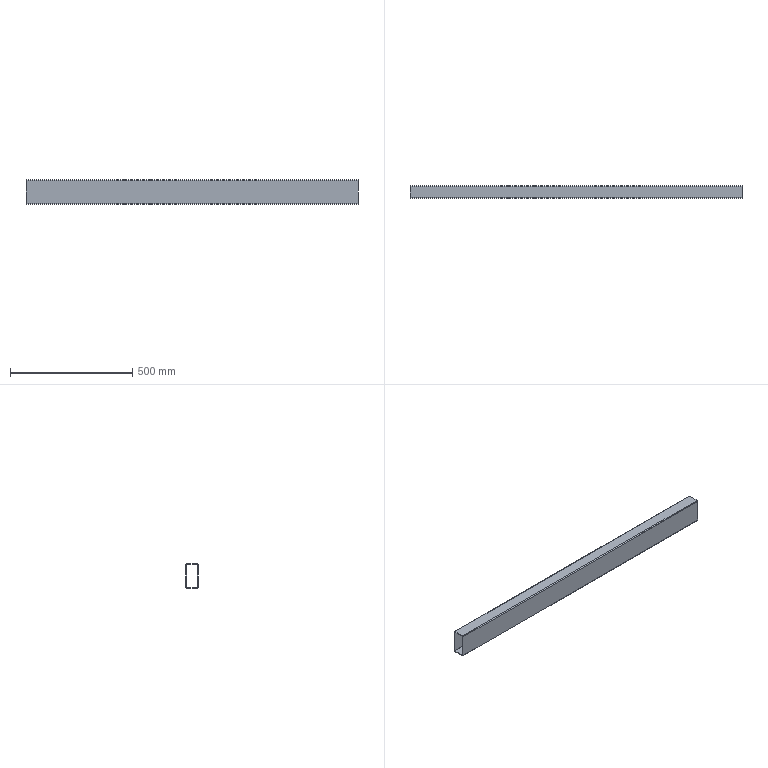Part | SolidWorks | features BaseBody 1, MoveFace 1 | 1 solid | 18 faces | box 1356 x 50 x 100 mm | volume 1157616 mm3 | plane 10 | cylinder 8 | commonest cylinder face diameters 1 x4 7 x4
STEP:
#1=CARTESIAN_POINT('',(976.,21.5,-50.));
#2=VERTEX_POINT('',#1);
#3=CARTESIAN_POINT('',(976.,25.,-46.5));
#4=VERTEX_POINT('',#3);
#5=CARTESIAN_POINT('',(976.,21.5,-46.5));
#6=DIRECTION('',(1.,0.,0.));
#7=DIRECTION('',(0.,0.,1.));
#8=AXIS2_PLACEMENT_3D('',#5,#6,#7);
#9=CIRCLE('',#8,3.5);
#10=EDGE_CURVE('',#2,#4,#9,.T.);
#11=ORIENTED_EDGE('',*,*,#10,.T.);
#12=CARTESIAN_POINT('',(976.,25.,46.5));
#13=VERTEX_POINT('',#12);
#14=CARTESIAN_POINT('',(976.,25.,46.5));
#15=DIRECTION('',(0.,0.,1.));
#16=VECTOR('',#15,1000.);
#17=LINE('',#14,#16);
#18=EDGE_CURVE('',#4,#13,#17,.T.);
#19=ORIENTED_EDGE('',*,*,#18,.T.);
#20=CARTESIAN_POINT('',(976.,21.5,50.));
#21=VERTEX_POINT('',#20);
#22=CARTESIAN_POINT('',(976.,21.5,46.5));
#23=DIRECTION('',(1.,0.,0.));
#24=DIRECTION('',(0.,0.,-1.));
#25=AXIS2_PLACEMENT_3D('',#22,#23,#24);
#26=CIRCLE('',#25,3.5);
#27=EDGE_CURVE('',#13,#21,#26,.T.);
#28=ORIENTED_EDGE('',*,*,#27,.T.);
#29=CARTESIAN_POINT('',(976.,-21.5,50.));
#30=VERTEX_POINT('',#29);
#31=CARTESIAN_POINT('',(976.,21.5,50.));
#32=DIRECTION('',(0.,-1.,0.));
#33=VECTOR('',#32,1000.);
#34=LINE('',#31,#33);
#35=EDGE_CURVE('',#21,#30,#34,.T.);
#36=ORIENTED_EDGE('',*,*,#35,.T.);
#37=CARTESIAN_POINT('',(976.,-25.,46.5));
#38=VERTEX_POINT('',#37);
#39=CARTESIAN_POINT('',(976.,-21.5,46.5));
#40=DIRECTION('',(1.,0.,0.));
#41=DIRECTION('',(0.,0.,-1.));
#42=AXIS2_PLACEMENT_3D('',#39,#40,#41);
#43=CIRCLE('',#42,3.5);
#44=EDGE_CURVE('',#30,#38,#43,.T.);
#45=ORIENTED_EDGE('',*,*,#44,.T.);
#46=CARTESIAN_POINT('',(976.,-25.,-46.5));
#47=VERTEX_POINT('',#46);
#48=CARTESIAN_POINT('',(976.,-25.,46.5));
#49=DIRECTION('',(0.,0.,-1.));
#50=VECTOR('',#49,1000.);
#51=LINE('',#48,#50);
#52=EDGE_CURVE('',#38,#47,#51,.T.);
#53=ORIENTED_EDGE('',*,*,#52,.T.);
#54=CARTESIAN_POINT('',(976.,-21.5,-50.));
#55=VERTEX_POINT('',#54);
#56=CARTESIAN_POINT('',(976.,-21.5,-46.5));
#57=DIRECTION('',(1.,0.,0.));
#58=DIRECTION('',(0.,0.,-1.));
#59=AXIS2_PLACEMENT_3D('',#56,#57,#58);
#60=CIRCLE('',#59,3.5);
#61=EDGE_CURVE('',#47,#55,#60,.T.);
#62=ORIENTED_EDGE('',*,*,#61,.T.);
#63=CARTESIAN_POINT('',(976.,21.5,-50.));
#64=DIRECTION('',(0.,1.,0.));
#65=VECTOR('',#64,1000.);
#66=LINE('',#63,#65);
#67=EDGE_CURVE('',#55,#2,#66,.T.);
#68=ORIENTED_EDGE('',*,*,#67,.T.);
#69=EDGE_LOOP('',(#11,#19,#28,#36,#45,#53,#62,#68));
#70=FACE_OUTER_BOUND('',#69,.T.);
#71=CARTESIAN_POINT('',(976.,22.,-46.5));
#72=VERTEX_POINT('',#71);
#73=CARTESIAN_POINT('',(976.,22.,46.5));
#74=VERTEX_POINT('',#73);
#75=CARTESIAN_POINT('',(976.,22.,-46.5));
#76=DIRECTION('',(0.,0.,1.));
#77=VECTOR('',#76,1000.);
#78=LINE('',#75,#77);
#79=EDGE_CURVE('',#72,#74,#78,.T.);
#80=ORIENTED_EDGE('',*,*,#79,.F.);
#81=CARTESIAN_POINT('',(976.,21.5,-47.));
#82=VERTEX_POINT('',#81);
#83=CARTESIAN_POINT('',(976.,21.5,-46.5));
#84=DIRECTION('',(1.,0.,0.));
#85=DIRECTION('',(0.,0.,1.));
#86=AXIS2_PLACEMENT_3D('',#83,#84,#85);
#87=CIRCLE('',#86,0.5);
#88=EDGE_CURVE('',#82,#72,#87,.T.);
#89=ORIENTED_EDGE('',*,*,#88,.F.);
#90=CARTESIAN_POINT('',(976.,-21.5,-47.));
#91=VERTEX_POINT('',#90);
#92=CARTESIAN_POINT('',(976.,21.5,-47.));
#93=DIRECTION('',(0.,1.,0.));
#94=VECTOR('',#93,1000.);
#95=LINE('',#92,#94);
#96=EDGE_CURVE('',#91,#82,#95,.T.);
#97=ORIENTED_EDGE('',*,*,#96,.F.);
#98=CARTESIAN_POINT('',(976.,-22.,-46.5));
#99=VERTEX_POINT('',#98);
#100=CARTESIAN_POINT('',(976.,-21.5,-46.5));
#101=DIRECTION('',(1.,0.,0.));
#102=DIRECTION('',(0.,0.,1.));
#103=AXIS2_PLACEMENT_3D('',#100,#101,#102);
#104=CIRCLE('',#103,0.5);
#105=EDGE_CURVE('',#99,#91,#104,.T.);
#106=ORIENTED_EDGE('',*,*,#105,.F.);
#107=CARTESIAN_POINT('',(976.,-22.,46.5));
#108=VERTEX_POINT('',#107);
#109=CARTESIAN_POINT('',(976.,-22.,-46.5));
#110=DIRECTION('',(0.,0.,-1.));
#111=VECTOR('',#110,1000.);
#112=LINE('',#109,#111);
#113=EDGE_CURVE('',#108,#99,#112,.T.);
#114=ORIENTED_EDGE('',*,*,#113,.F.);
#115=CARTESIAN_POINT('',(976.,-21.5,47.));
#116=VERTEX_POINT('',#115);
#117=CARTESIAN_POINT('',(976.,-21.5,46.5));
#118=DIRECTION('',(1.,0.,0.));
#119=DIRECTION('',(0.,0.,1.));
#120=AXIS2_PLACEMENT_3D('',#117,#118,#119);
#121=CIRCLE('',#120,0.5);
#122=EDGE_CURVE('',#116,#108,#121,.T.);
#123=ORIENTED_EDGE('',*,*,#122,.F.);
#124=CARTESIAN_POINT('',(976.,21.5,47.));
#125=VERTEX_POINT('',#124);
#126=CARTESIAN_POINT('',(976.,21.5,47.));
#127=DIRECTION('',(0.,-1.,0.));
#128=VECTOR('',#127,1000.);
#129=LINE('',#126,#128);
#130=EDGE_CURVE('',#125,#116,#129,.T.);
#131=ORIENTED_EDGE('',*,*,#130,.F.);
#132=CARTESIAN_POINT('',(976.,21.5,46.5));
#133=DIRECTION('',(1.,0.,0.));
#134=DIRECTION('',(0.,0.,1.));
#135=AXIS2_PLACEMENT_3D('',#132,#133,#134);
#136=CIRCLE('',#135,0.5);
#137=EDGE_CURVE('',#74,#125,#136,.T.);
#138=ORIENTED_EDGE('',*,*,#137,.F.);
#139=EDGE_LOOP('',(#80,#89,#97,#106,#114,#123,#131,#138));
#140=FACE_BOUND('',#139,.T.);
#141=CARTESIAN_POINT('',(976.,21.5,-46.5));
#142=DIRECTION('',(1.,0.,0.));
#143=DIRECTION('',(0.,0.,-1.));
#144=AXIS2_PLACEMENT_3D('',#141,#142,#143);
#145=PLANE('',#144);
#146=ADVANCED_FACE('',(#70,#140),#145,.T.);
#147=CARTESIAN_POINT('',(-380.,21.5,-50.));
#148=VERTEX_POINT('',#147);
#149=CARTESIAN_POINT('',(-380.,25.,-46.5));
#150=VERTEX_POINT('',#149);
#151=CARTESIAN_POINT('',(-380.,21.5,-46.5));
#152=DIRECTION('',(1.,0.,0.));
#153=DIRECTION('',(0.,0.,1.));
#154=AXIS2_PLACEMENT_3D('',#151,#152,#153);
#155=CIRCLE('',#154,3.5);
#156=EDGE_CURVE('',#148,#150,#155,.T.);
#157=ORIENTED_EDGE('',*,*,#156,.F.);
#158=CARTESIAN_POINT('',(-380.,-21.5,-50.));
#159=VERTEX_POINT('',#158);
#160=CARTESIAN_POINT('',(-380.,21.5,-50.));
#161=DIRECTION('',(0.,1.,0.));
#162=VECTOR('',#161,1000.);
#163=LINE('',#160,#162);
#164=EDGE_CURVE('',#159,#148,#163,.T.);
#165=ORIENTED_EDGE('',*,*,#164,.F.);
#166=CARTESIAN_POINT('',(-380.,-25.,-46.5));
#167=VERTEX_POINT('',#166);
#168=CARTESIAN_POINT('',(-380.,-21.5,-46.5));
#169=DIRECTION('',(1.,0.,0.));
#170=DIRECTION('',(0.,0.,-1.));
#171=AXIS2_PLACEMENT_3D('',#168,#169,#170);
#172=CIRCLE('',#171,3.5);
#173=EDGE_CURVE('',#167,#159,#172,.T.);
#174=ORIENTED_EDGE('',*,*,#173,.F.);
#175=CARTESIAN_POINT('',(-380.,-25.,46.5));
#176=VERTEX_POINT('',#175);
#177=CARTESIAN_POINT('',(-380.,-25.,46.5));
#178=DIRECTION('',(0.,0.,-1.));
#179=VECTOR('',#178,1000.);
#180=LINE('',#177,#179);
#181=EDGE_CURVE('',#176,#167,#180,.T.);
#182=ORIENTED_EDGE('',*,*,#181,.F.);
#183=CARTESIAN_POINT('',(-380.,-21.5,50.));
#184=VERTEX_POINT('',#183);
#185=CARTESIAN_POINT('',(-380.,-21.5,46.5));
#186=DIRECTION('',(1.,0.,0.));
#187=DIRECTION('',(0.,0.,-1.));
#188=AXIS2_PLACEMENT_3D('',#185,#186,#187);
#189=CIRCLE('',#188,3.5);
#190=EDGE_CURVE('',#184,#176,#189,.T.);
#191=ORIENTED_EDGE('',*,*,#190,.F.);
#192=CARTESIAN_POINT('',(-380.,21.5,50.));
#193=VERTEX_POINT('',#192);
#194=CARTESIAN_POINT('',(-380.,21.5,50.));
#195=DIRECTION('',(0.,-1.,0.));
#196=VECTOR('',#195,1000.);
#197=LINE('',#194,#196);
#198=EDGE_CURVE('',#193,#184,#197,.T.);
#199=ORIENTED_EDGE('',*,*,#198,.F.);
#200=CARTESIAN_POINT('',(-380.,25.,46.5));
#201=VERTEX_POINT('',#200);
#202=CARTESIAN_POINT('',(-380.,21.5,46.5));
#203=DIRECTION('',(1.,0.,0.));
#204=DIRECTION('',(0.,0.,-1.));
#205=AXIS2_PLACEMENT_3D('',#202,#203,#204);
#206=CIRCLE('',#205,3.5);
#207=EDGE_CURVE('',#201,#193,#206,.T.);
#208=ORIENTED_EDGE('',*,*,#207,.F.);
#209=CARTESIAN_POINT('',(-380.,25.,46.5));
#210=DIRECTION('',(0.,0.,1.));
#211=VECTOR('',#210,1000.);
#212=LINE('',#209,#211);
#213=EDGE_CURVE('',#150,#201,#212,.T.);
#214=ORIENTED_EDGE('',*,*,#213,.F.);
#215=EDGE_LOOP('',(#157,#165,#174,#182,#191,#199,#208,#214));
#216=FACE_OUTER_BOUND('',#215,.T.);
#217=CARTESIAN_POINT('',(-380.,21.5,-47.));
#218=VERTEX_POINT('',#217);
#219=CARTESIAN_POINT('',(-380.,22.,-46.5));
#220=VERTEX_POINT('',#219);
#221=CARTESIAN_POINT('',(-380.,21.5,-46.5));
#222=DIRECTION('',(1.,0.,0.));
#223=DIRECTION('',(0.,0.,1.));
#224=AXIS2_PLACEMENT_3D('',#221,#222,#223);
#225=CIRCLE('',#224,0.5);
#226=EDGE_CURVE('',#218,#220,#225,.T.);
#227=ORIENTED_EDGE('',*,*,#226,.T.);
#228=CARTESIAN_POINT('',(-380.,22.,46.5));
#229=VERTEX_POINT('',#228);
#230=CARTESIAN_POINT('',(-380.,22.,-46.5));
#231=DIRECTION('',(0.,0.,1.));
#232=VECTOR('',#231,1000.);
#233=LINE('',#230,#232);
#234=EDGE_CURVE('',#220,#229,#233,.T.);
#235=ORIENTED_EDGE('',*,*,#234,.T.);
#236=CARTESIAN_POINT('',(-380.,21.5,47.));
#237=VERTEX_POINT('',#236);
#238=CARTESIAN_POINT('',(-380.,21.5,46.5));
#239=DIRECTION('',(1.,0.,0.));
#240=DIRECTION('',(0.,0.,1.));
#241=AXIS2_PLACEMENT_3D('',#238,#239,#240);
#242=CIRCLE('',#241,0.5);
#243=EDGE_CURVE('',#229,#237,#242,.T.);
#244=ORIENTED_EDGE('',*,*,#243,.T.);
#245=CARTESIAN_POINT('',(-380.,-21.5,47.));
#246=VERTEX_POINT('',#245);
#247=CARTESIAN_POINT('',(-380.,21.5,47.));
#248=DIRECTION('',(0.,-1.,0.));
#249=VECTOR('',#248,1000.);
#250=LINE('',#247,#249);
#251=EDGE_CURVE('',#237,#246,#250,.T.);
#252=ORIENTED_EDGE('',*,*,#251,.T.);
#253=CARTESIAN_POINT('',(-380.,-22.,46.5));
#254=VERTEX_POINT('',#253);
#255=CARTESIAN_POINT('',(-380.,-21.5,46.5));
#256=DIRECTION('',(1.,0.,0.));
#257=DIRECTION('',(0.,0.,1.));
#258=AXIS2_PLACEMENT_3D('',#255,#256,#257);
#259=CIRCLE('',#258,0.5);
#260=EDGE_CURVE('',#246,#254,#259,.T.);
#261=ORIENTED_EDGE('',*,*,#260,.T.);
#262=CARTESIAN_POINT('',(-380.,-22.,-46.5));
#263=VERTEX_POINT('',#262);
#264=CARTESIAN_POINT('',(-380.,-22.,-46.5));
#265=DIRECTION('',(0.,0.,-1.));
#266=VECTOR('',#265,1000.);
#267=LINE('',#264,#266);
#268=EDGE_CURVE('',#254,#263,#267,.T.);
#269=ORIENTED_EDGE('',*,*,#268,.T.);
#270=CARTESIAN_POINT('',(-380.,-21.5,-47.));
#271=VERTEX_POINT('',#270);
#272=CARTESIAN_POINT('',(-380.,-21.5,-46.5));
#273=DIRECTION('',(1.,0.,0.));
#274=DIRECTION('',(0.,0.,1.));
#275=AXIS2_PLACEMENT_3D('',#272,#273,#274);
#276=CIRCLE('',#275,0.5);
#277=EDGE_CURVE('',#263,#271,#276,.T.);
#278=ORIENTED_EDGE('',*,*,#277,.T.);
#279=CARTESIAN_POINT('',(-380.,21.5,-47.));
#280=DIRECTION('',(0.,1.,0.));
#281=VECTOR('',#280,1000.);
#282=LINE('',#279,#281);
#283=EDGE_CURVE('',#271,#218,#282,.T.);
#284=ORIENTED_EDGE('',*,*,#283,.T.);
#285=EDGE_LOOP('',(#227,#235,#244,#252,#261,#269,#278,#284));
#286=FACE_BOUND('',#285,.T.);
#287=CARTESIAN_POINT('',(-380.,21.5,-46.5));
#288=DIRECTION('',(1.,0.,0.));
#289=DIRECTION('',(0.,0.,-1.));
#290=AXIS2_PLACEMENT_3D('',#287,#288,#289);
#291=PLANE('',#290);
#292=ADVANCED_FACE('',(#216,#286),#291,.F.);
#293=ORIENTED_EDGE('',*,*,#156,.T.);
#294=CARTESIAN_POINT('',(976.,25.,-46.5));
#295=DIRECTION('',(-1.,0.,0.));
#296=VECTOR('',#295,1000.);
#297=LINE('',#294,#296);
#298=EDGE_CURVE('',#4,#150,#297,.T.);
#299=ORIENTED_EDGE('',*,*,#298,.F.);
#300=ORIENTED_EDGE('',*,*,#10,.F.);
#301=CARTESIAN_POINT('',(976.,21.5,-50.));
#302=DIRECTION('',(-1.,0.,0.));
#303=VECTOR('',#302,1000.);
#304=LINE('',#301,#303);
#305=EDGE_CURVE('',#2,#148,#304,.T.);
#306=ORIENTED_EDGE('',*,*,#305,.T.);
#307=EDGE_LOOP('',(#293,#299,#300,#306));
#308=FACE_OUTER_BOUND('',#307,.T.);
#309=CARTESIAN_POINT('',(976.,21.5,-46.5));
#310=DIRECTION('',(-1.,0.,0.));
#311=DIRECTION('',(0.,0.,1.));
#312=AXIS2_PLACEMENT_3D('',#309,#310,#311);
#313=CYLINDRICAL_SURFACE('',#312,3.5);
#314=ADVANCED_FACE('',(#308),#313,.T.);
#315=ORIENTED_EDGE('',*,*,#213,.T.);
#316=CARTESIAN_POINT('',(976.,25.,46.5));
#317=DIRECTION('',(-1.,0.,0.));
#318=VECTOR('',#317,1000.);
#319=LINE('',#316,#318);
#320=EDGE_CURVE('',#13,#201,#319,.T.);
#321=ORIENTED_EDGE('',*,*,#320,.F.);
#322=ORIENTED_EDGE('',*,*,#18,.F.);
#323=ORIENTED_EDGE('',*,*,#298,.T.);
#324=EDGE_LOOP('',(#315,#321,#322,#323));
#325=FACE_OUTER_BOUND('',#324,.T.);
#326=CARTESIAN_POINT('',(976.,25.,46.5));
#327=DIRECTION('',(0.,-1.,0.));
#328=DIRECTION('',(0.,0.,-1.));
#329=AXIS2_PLACEMENT_3D('',#326,#327,#328);
#330=PLANE('',#329);
#331=ADVANCED_FACE('',(#325),#330,.F.);
#332=ORIENTED_EDGE('',*,*,#207,.T.);
#333=CARTESIAN_POINT('',(976.,21.5,50.));
#334=DIRECTION('',(-1.,0.,0.));
#335=VECTOR('',#334,1000.);
#336=LINE('',#333,#335);
#337=EDGE_CURVE('',#21,#193,#336,.T.);
#338=ORIENTED_EDGE('',*,*,#337,.F.);
#339=ORIENTED_EDGE('',*,*,#27,.F.);
#340=ORIENTED_EDGE('',*,*,#320,.T.);
#341=EDGE_LOOP('',(#332,#338,#339,#340));
#342=FACE_OUTER_BOUND('',#341,.T.);
#343=CARTESIAN_POINT('',(976.,21.5,46.5));
#344=DIRECTION('',(-1.,0.,0.));
#345=DIRECTION('',(0.,0.,1.));
#346=AXIS2_PLACEMENT_3D('',#343,#344,#345);
#347=CYLINDRICAL_SURFACE('',#346,3.5);
#348=ADVANCED_FACE('',(#342),#347,.T.);
#349=ORIENTED_EDGE('',*,*,#198,.T.);
#350=CARTESIAN_POINT('',(976.,-21.5,50.));
#351=DIRECTION('',(-1.,0.,0.));
#352=VECTOR('',#351,1000.);
#353=LINE('',#350,#352);
#354=EDGE_CURVE('',#30,#184,#353,.T.);
#355=ORIENTED_EDGE('',*,*,#354,.F.);
#356=ORIENTED_EDGE('',*,*,#35,.F.);
#357=ORIENTED_EDGE('',*,*,#337,.T.);
#358=EDGE_LOOP('',(#349,#355,#356,#357));
#359=FACE_OUTER_BOUND('',#358,.T.);
#360=CARTESIAN_POINT('',(976.,21.5,50.));
#361=DIRECTION('',(0.,0.,-1.));
#362=DIRECTION('',(-1.,0.,0.));
#363=AXIS2_PLACEMENT_3D('',#360,#361,#362);
#364=PLANE('',#363);
#365=ADVANCED_FACE('',(#359),#364,.F.);
#366=ORIENTED_EDGE('',*,*,#190,.T.);
#367=CARTESIAN_POINT('',(976.,-25.,46.5));
#368=DIRECTION('',(-1.,0.,0.));
#369=VECTOR('',#368,1000.);
#370=LINE('',#367,#369);
#371=EDGE_CURVE('',#38,#176,#370,.T.);
#372=ORIENTED_EDGE('',*,*,#371,.F.);
#373=ORIENTED_EDGE('',*,*,#44,.F.);
#374=ORIENTED_EDGE('',*,*,#354,.T.);
#375=EDGE_LOOP('',(#366,#372,#373,#374));
#376=FACE_OUTER_BOUND('',#375,.T.);
#377=CARTESIAN_POINT('',(976.,-21.5,46.5));
#378=DIRECTION('',(-1.,0.,0.));
#379=DIRECTION('',(0.,0.,1.));
#380=AXIS2_PLACEMENT_3D('',#377,#378,#379);
#381=CYLINDRICAL_SURFACE('',#380,3.5);
#382=ADVANCED_FACE('',(#376),#381,.T.);
#383=ORIENTED_EDGE('',*,*,#181,.T.);
#384=CARTESIAN_POINT('',(976.,-25.,-46.5));
#385=DIRECTION('',(-1.,0.,0.));
#386=VECTOR('',#385,1000.);
#387=LINE('',#384,#386);
#388=EDGE_CURVE('',#47,#167,#387,.T.);
#389=ORIENTED_EDGE('',*,*,#388,.F.);
#390=ORIENTED_EDGE('',*,*,#52,.F.);
#391=ORIENTED_EDGE('',*,*,#371,.T.);
#392=EDGE_LOOP('',(#383,#389,#390,#391));
#393=FACE_OUTER_BOUND('',#392,.T.);
#394=CARTESIAN_POINT('',(976.,-25.,46.5));
#395=DIRECTION('',(0.,1.,0.));
#396=DIRECTION('',(0.,0.,1.));
#397=AXIS2_PLACEMENT_3D('',#394,#395,#396);
#398=PLANE('',#397);
#399=ADVANCED_FACE('',(#393),#398,.F.);
#400=ORIENTED_EDGE('',*,*,#173,.T.);
#401=CARTESIAN_POINT('',(976.,-21.5,-50.));
#402=DIRECTION('',(-1.,0.,0.));
#403=VECTOR('',#402,1000.);
#404=LINE('',#401,#403);
#405=EDGE_CURVE('',#55,#159,#404,.T.);
#406=ORIENTED_EDGE('',*,*,#405,.F.);
#407=ORIENTED_EDGE('',*,*,#61,.F.);
#408=ORIENTED_EDGE('',*,*,#388,.T.);
#409=EDGE_LOOP('',(#400,#406,#407,#408));
#410=FACE_OUTER_BOUND('',#409,.T.);
#411=CARTESIAN_POINT('',(976.,-21.5,-46.5));
#412=DIRECTION('',(-1.,0.,0.));
#413=DIRECTION('',(0.,0.,1.));
#414=AXIS2_PLACEMENT_3D('',#411,#412,#413);
#415=CYLINDRICAL_SURFACE('',#414,3.5);
#416=ADVANCED_FACE('',(#410),#415,.T.);
#417=ORIENTED_EDGE('',*,*,#164,.T.);
#418=ORIENTED_EDGE('',*,*,#305,.F.);
#419=ORIENTED_EDGE('',*,*,#67,.F.);
#420=ORIENTED_EDGE('',*,*,#405,.T.);
#421=EDGE_LOOP('',(#417,#418,#419,#420));
#422=FACE_OUTER_BOUND('',#421,.T.);
#423=CARTESIAN_POINT('',(976.,21.5,-50.));
#424=DIRECTION('',(0.,0.,1.));
#425=DIRECTION('',(0.,-1.,0.));
#426=AXIS2_PLACEMENT_3D('',#423,#424,#425);
#427=PLANE('',#426);
#428=ADVANCED_FACE('',(#422),#427,.F.);
#429=ORIENTED_EDGE('',*,*,#226,.F.);
#430=CARTESIAN_POINT('',(976.,21.5,-47.));
#431=DIRECTION('',(-1.,0.,0.));
#432=VECTOR('',#431,1000.);
#433=LINE('',#430,#432);
#434=EDGE_CURVE('',#82,#218,#433,.T.);
#435=ORIENTED_EDGE('',*,*,#434,.F.);
#436=ORIENTED_EDGE('',*,*,#88,.T.);
#437=CARTESIAN_POINT('',(976.,22.,-46.5));
#438=DIRECTION('',(-1.,0.,0.));
#439=VECTOR('',#438,1000.);
#440=LINE('',#437,#439);
#441=EDGE_CURVE('',#72,#220,#440,.T.);
#442=ORIENTED_EDGE('',*,*,#441,.T.);
#443=EDGE_LOOP('',(#429,#435,#436,#442));
#444=FACE_OUTER_BOUND('',#443,.T.);
#445=CARTESIAN_POINT('',(976.,21.5,-46.5));
#446=DIRECTION('',(-1.,0.,0.));
#447=DIRECTION('',(0.,0.,1.));
#448=AXIS2_PLACEMENT_3D('',#445,#446,#447);
#449=CYLINDRICAL_SURFACE('',#448,0.5);
#450=ADVANCED_FACE('',(#444),#449,.F.);
#451=ORIENTED_EDGE('',*,*,#234,.F.);
#452=ORIENTED_EDGE('',*,*,#441,.F.);
#453=ORIENTED_EDGE('',*,*,#79,.T.);
#454=CARTESIAN_POINT('',(976.,22.,46.5));
#455=DIRECTION('',(-1.,0.,0.));
#456=VECTOR('',#455,1000.);
#457=LINE('',#454,#456);
#458=EDGE_CURVE('',#74,#229,#457,.T.);
#459=ORIENTED_EDGE('',*,*,#458,.T.);
#460=EDGE_LOOP('',(#451,#452,#453,#459));
#461=FACE_OUTER_BOUND('',#460,.T.);
#462=CARTESIAN_POINT('',(976.,22.,-46.5));
#463=DIRECTION('',(0.,-1.,0.));
#464=DIRECTION('',(0.,0.,-1.));
#465=AXIS2_PLACEMENT_3D('',#462,#463,#464);
#466=PLANE('',#465);
#467=ADVANCED_FACE('',(#461),#466,.T.);
#468=ORIENTED_EDGE('',*,*,#243,.F.);
#469=ORIENTED_EDGE('',*,*,#458,.F.);
#470=ORIENTED_EDGE('',*,*,#137,.T.);
#471=CARTESIAN_POINT('',(976.,21.5,47.));
#472=DIRECTION('',(-1.,0.,0.));
#473=VECTOR('',#472,1000.);
#474=LINE('',#471,#473);
#475=EDGE_CURVE('',#125,#237,#474,.T.);
#476=ORIENTED_EDGE('',*,*,#475,.T.);
#477=EDGE_LOOP('',(#468,#469,#470,#476));
#478=FACE_OUTER_BOUND('',#477,.T.);
#479=CARTESIAN_POINT('',(976.,21.5,46.5));
#480=DIRECTION('',(-1.,0.,0.));
#481=DIRECTION('',(0.,0.,1.));
#482=AXIS2_PLACEMENT_3D('',#479,#480,#481);
#483=CYLINDRICAL_SURFACE('',#482,0.5);
#484=ADVANCED_FACE('',(#478),#483,.F.);
#485=ORIENTED_EDGE('',*,*,#251,.F.);
#486=ORIENTED_EDGE('',*,*,#475,.F.);
#487=ORIENTED_EDGE('',*,*,#130,.T.);
#488=CARTESIAN_POINT('',(976.,-21.5,47.));
#489=DIRECTION('',(-1.,0.,0.));
#490=VECTOR('',#489,1000.);
#491=LINE('',#488,#490);
#492=EDGE_CURVE('',#116,#246,#491,.T.);
#493=ORIENTED_EDGE('',*,*,#492,.T.);
#494=EDGE_LOOP('',(#485,#486,#487,#493));
#495=FACE_OUTER_BOUND('',#494,.T.);
#496=CARTESIAN_POINT('',(976.,21.5,47.));
#497=DIRECTION('',(0.,0.,-1.));
#498=DIRECTION('',(-1.,0.,0.));
#499=AXIS2_PLACEMENT_3D('',#496,#497,#498);
#500=PLANE('',#499);
#501=ADVANCED_FACE('',(#495),#500,.T.);
#502=ORIENTED_EDGE('',*,*,#260,.F.);
#503=ORIENTED_EDGE('',*,*,#492,.F.);
#504=ORIENTED_EDGE('',*,*,#122,.T.);
#505=CARTESIAN_POINT('',(976.,-22.,46.5));
#506=DIRECTION('',(-1.,0.,0.));
#507=VECTOR('',#506,1000.);
#508=LINE('',#505,#507);
#509=EDGE_CURVE('',#108,#254,#508,.T.);
#510=ORIENTED_EDGE('',*,*,#509,.T.);
#511=EDGE_LOOP('',(#502,#503,#504,#510));
#512=FACE_OUTER_BOUND('',#511,.T.);
#513=CARTESIAN_POINT('',(976.,-21.5,46.5));
#514=DIRECTION('',(-1.,0.,0.));
#515=DIRECTION('',(0.,0.,1.));
#516=AXIS2_PLACEMENT_3D('',#513,#514,#515);
#517=CYLINDRICAL_SURFACE('',#516,0.5);
#518=ADVANCED_FACE('',(#512),#517,.F.);
#519=ORIENTED_EDGE('',*,*,#268,.F.);
#520=ORIENTED_EDGE('',*,*,#509,.F.);
#521=ORIENTED_EDGE('',*,*,#113,.T.);
#522=CARTESIAN_POINT('',(976.,-22.,-46.5));
#523=DIRECTION('',(-1.,0.,0.));
#524=VECTOR('',#523,1000.);
#525=LINE('',#522,#524);
#526=EDGE_CURVE('',#99,#263,#525,.T.);
#527=ORIENTED_EDGE('',*,*,#526,.T.);
#528=EDGE_LOOP('',(#519,#520,#521,#527));
#529=FACE_OUTER_BOUND('',#528,.T.);
#530=CARTESIAN_POINT('',(976.,-22.,-46.5));
#531=DIRECTION('',(0.,1.,0.));
#532=DIRECTION('',(0.,0.,1.));
#533=AXIS2_PLACEMENT_3D('',#530,#531,#532);
#534=PLANE('',#533);
#535=ADVANCED_FACE('',(#529),#534,.T.);
#536=ORIENTED_EDGE('',*,*,#277,.F.);
#537=ORIENTED_EDGE('',*,*,#526,.F.);
#538=ORIENTED_EDGE('',*,*,#105,.T.);
#539=CARTESIAN_POINT('',(976.,-21.5,-47.));
#540=DIRECTION('',(-1.,0.,0.));
#541=VECTOR('',#540,1000.);
#542=LINE('',#539,#541);
#543=EDGE_CURVE('',#91,#271,#542,.T.);
#544=ORIENTED_EDGE('',*,*,#543,.T.);
#545=EDGE_LOOP('',(#536,#537,#538,#544));
#546=FACE_OUTER_BOUND('',#545,.T.);
#547=CARTESIAN_POINT('',(976.,-21.5,-46.5));
#548=DIRECTION('',(-1.,0.,0.));
#549=DIRECTION('',(0.,0.,1.));
#550=AXIS2_PLACEMENT_3D('',#547,#548,#549);
#551=CYLINDRICAL_SURFACE('',#550,0.5);
#552=ADVANCED_FACE('',(#546),#551,.F.);
#553=ORIENTED_EDGE('',*,*,#283,.F.);
#554=ORIENTED_EDGE('',*,*,#543,.F.);
#555=ORIENTED_EDGE('',*,*,#96,.T.);
#556=ORIENTED_EDGE('',*,*,#434,.T.);
#557=EDGE_LOOP('',(#553,#554,#555,#556));
#558=FACE_OUTER_BOUND('',#557,.T.);
#559=CARTESIAN_POINT('',(976.,21.5,-47.));
#560=DIRECTION('',(0.,0.,1.));
#561=DIRECTION('',(0.,-1.,0.));
#562=AXIS2_PLACEMENT_3D('',#559,#560,#561);
#563=PLANE('',#562);
#564=ADVANCED_FACE('',(#558),#563,.T.);
#565=CLOSED_SHELL('',(#146,#292,#314,#331,#348,#365,#382,#399,#416,#428,#450,#467,#484,#501,#518,#535,#552,#564));
#566=MANIFOLD_SOLID_BREP('',#565);
#567=CARTESIAN_POINT('',(0.,0.,0.));
#568=DIRECTION('',(0.,0.,1.));
#569=DIRECTION('',(1.,0.,0.));
#570=AXIS2_PLACEMENT_3D('',#567,#568,#569);
#571=(LENGTH_UNIT()NAMED_UNIT(*)SI_UNIT(.MILLI.,.METRE.));
#572=UNCERTAINTY_MEASURE_WITH_UNIT(LENGTH_MEASURE(0.00001),#571,'','');
#573=(NAMED_UNIT(*)PLANE_ANGLE_UNIT()SI_UNIT($,.RADIAN.));
#574=(NAMED_UNIT(*)SI_UNIT($,.STERADIAN.)SOLID_ANGLE_UNIT());
#575=(GEOMETRIC_REPRESENTATION_CONTEXT(3)GLOBAL_UNCERTAINTY_ASSIGNED_CONTEXT((#572))GLOBAL_UNIT_ASSIGNED_CONTEXT((#571,#573,#574))REPRESENTATION_CONTEXT('',''));
#576=ADVANCED_BREP_SHAPE_REPRESENTATION('',(#566,#570),#575);